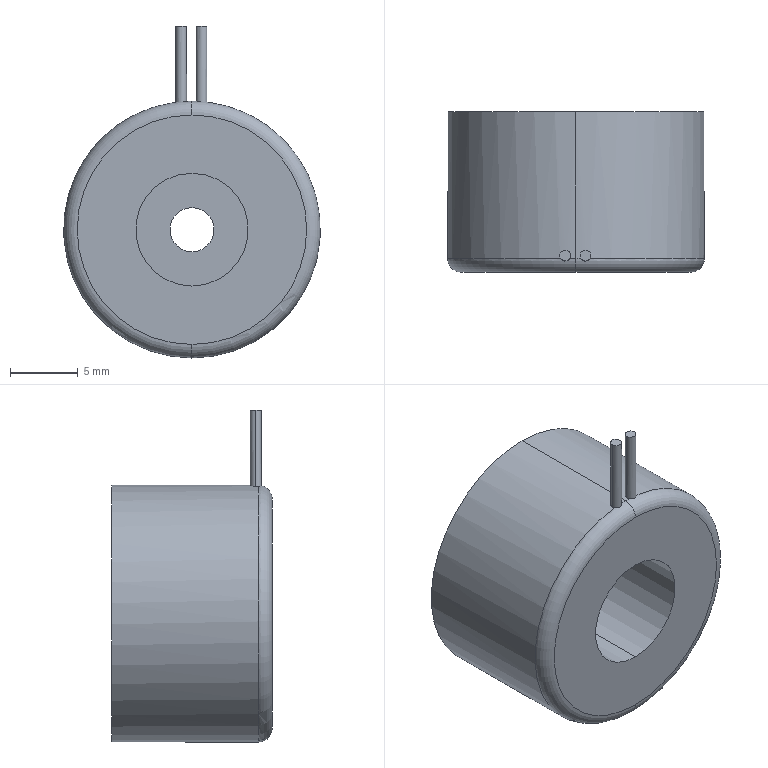Part | SolidWorks | features ICE 2, HoleWzd 1, Revolution 1 | 1 solid | 25 faces | box 18.9 x 11.8 x 24.45 mm | volume 2887 mm3 | cylinder 14 | plane 5 | cone 4 | torus 2 | commonest cylinder face diameters 0.8 x4 2.05 x4 3.25 x2 8.3 x2 18.9 x2
STEP:
#1=CARTESIAN_POINT('',(1.1,1.2,15.));
#2=VERTEX_POINT('',#1);
#3=CARTESIAN_POINT('',(0.3,1.2,15.));
#4=VERTEX_POINT('',#3);
#5=CARTESIAN_POINT('',(0.7,1.2,15.));
#6=DIRECTION('',(0.,0.,1.));
#7=DIRECTION('',(1.,0.,0.));
#8=AXIS2_PLACEMENT_3D('',#5,#6,#7);
#9=CIRCLE('',#8,0.4);
#10=EDGE_CURVE('',#2,#4,#9,.T.);
#11=ORIENTED_EDGE('',*,*,#10,.F.);
#12=CARTESIAN_POINT('',(1.1,1.2,9.386));
#13=VERTEX_POINT('',#12);
#14=CARTESIAN_POINT('',(1.1,1.2,15.));
#15=DIRECTION('',(0.,0.,-1.));
#16=VECTOR('',#15,1000.);
#17=LINE('',#14,#16);
#18=EDGE_CURVE('',#2,#13,#17,.T.);
#19=ORIENTED_EDGE('',*,*,#18,.T.);
#20=CARTESIAN_POINT('',(0.3,1.2,9.445));
#21=VERTEX_POINT('',#20);
#22=CARTESIAN_POINT('',(0.3,1.2,9.445));
#23=CARTESIAN_POINT('',(0.3,1.306,9.445));
#24=CARTESIAN_POINT('',(0.3435,1.409,9.444));
#25=CARTESIAN_POINT('',(0.4915,1.557,9.438));
#26=CARTESIAN_POINT('',(0.596,1.6,9.432));
#27=CARTESIAN_POINT('',(0.8045,1.6,9.416));
#28=CARTESIAN_POINT('',(0.9081,1.558,9.407));
#29=CARTESIAN_POINT('',(1.057,1.408,9.391));
#30=CARTESIAN_POINT('',(1.1,1.305,9.386));
#31=CARTESIAN_POINT('',(1.1,1.2,9.386));
#32=B_SPLINE_CURVE_WITH_KNOTS('',3,(#22,#23,#24,#25,#26,#27,#28,#29,#30,#31),.UNSPECIFIED.,.F.,.F.,(4,2,2,2,4),(0.,0.0003131,0.0006262,0.0009394,0.001252),.UNSPECIFIED.);
#33=EDGE_CURVE('',#21,#13,#32,.T.);
#34=ORIENTED_EDGE('',*,*,#33,.F.);
#35=CARTESIAN_POINT('',(0.3,1.2,15.));
#36=DIRECTION('',(0.,0.,-1.));
#37=VECTOR('',#36,1000.);
#38=LINE('',#35,#37);
#39=EDGE_CURVE('',#4,#21,#38,.T.);
#40=ORIENTED_EDGE('',*,*,#39,.F.);
#41=EDGE_LOOP('',(#11,#19,#34,#40));
#42=FACE_OUTER_BOUND('',#41,.T.);
#43=CARTESIAN_POINT('',(0.7,1.2,15.));
#44=DIRECTION('',(0.,0.,-1.));
#45=DIRECTION('',(-1.,0.,0.));
#46=AXIS2_PLACEMENT_3D('',#43,#44,#45);
#47=CYLINDRICAL_SURFACE('',#46,0.4);
#48=ADVANCED_FACE('',(#42),#47,.T.);
#49=CARTESIAN_POINT('',(-0.4,1.2,15.));
#50=VERTEX_POINT('',#49);
#51=CARTESIAN_POINT('',(-1.2,1.2,15.));
#52=VERTEX_POINT('',#51);
#53=CARTESIAN_POINT('',(-0.8,1.2,15.));
#54=DIRECTION('',(0.,0.,1.));
#55=DIRECTION('',(1.,0.,0.));
#56=AXIS2_PLACEMENT_3D('',#53,#54,#55);
#57=CIRCLE('',#56,0.4);
#58=EDGE_CURVE('',#50,#52,#57,.T.);
#59=ORIENTED_EDGE('',*,*,#58,.F.);
#60=CARTESIAN_POINT('',(-0.4,1.2,9.442));
#61=VERTEX_POINT('',#60);
#62=CARTESIAN_POINT('',(-0.4,1.2,15.));
#63=DIRECTION('',(0.,0.,-1.));
#64=VECTOR('',#63,1000.);
#65=LINE('',#62,#64);
#66=EDGE_CURVE('',#50,#61,#65,.T.);
#67=ORIENTED_EDGE('',*,*,#66,.T.);
#68=CARTESIAN_POINT('',(-1.2,1.2,9.373));
#69=VERTEX_POINT('',#68);
#70=CARTESIAN_POINT('',(-1.2,1.2,9.373));
#71=CARTESIAN_POINT('',(-1.2,1.306,9.373));
#72=CARTESIAN_POINT('',(-1.156,1.409,9.379));
#73=CARTESIAN_POINT('',(-1.009,1.557,9.396));
#74=CARTESIAN_POINT('',(-0.9048,1.6,9.407));
#75=CARTESIAN_POINT('',(-0.6964,1.6,9.425));
#76=CARTESIAN_POINT('',(-0.5925,1.558,9.432));
#77=CARTESIAN_POINT('',(-0.4427,1.409,9.44));
#78=CARTESIAN_POINT('',(-0.4,1.305,9.442));
#79=CARTESIAN_POINT('',(-0.4,1.2,9.442));
#80=B_SPLINE_CURVE_WITH_KNOTS('',3,(#70,#71,#72,#73,#74,#75,#76,#77,#78,#79),.UNSPECIFIED.,.F.,.F.,(4,2,2,2,4),(0.,0.0003133,0.0006265,0.0009398,0.001253),.UNSPECIFIED.);
#81=EDGE_CURVE('',#69,#61,#80,.T.);
#82=ORIENTED_EDGE('',*,*,#81,.F.);
#83=CARTESIAN_POINT('',(-1.2,1.2,15.));
#84=DIRECTION('',(0.,0.,-1.));
#85=VECTOR('',#84,1000.);
#86=LINE('',#83,#85);
#87=EDGE_CURVE('',#52,#69,#86,.T.);
#88=ORIENTED_EDGE('',*,*,#87,.F.);
#89=EDGE_LOOP('',(#59,#67,#82,#88));
#90=FACE_OUTER_BOUND('',#89,.T.);
#91=CARTESIAN_POINT('',(-0.8,1.2,15.));
#92=DIRECTION('',(0.,0.,-1.));
#93=DIRECTION('',(-1.,0.,0.));
#94=AXIS2_PLACEMENT_3D('',#91,#92,#93);
#95=CYLINDRICAL_SURFACE('',#94,0.4);
#96=ADVANCED_FACE('',(#90),#95,.T.);
#97=CARTESIAN_POINT('',(0.,7.45,-7.275));
#98=VERTEX_POINT('',#97);
#99=CARTESIAN_POINT('',(0.,7.45,-5.225));
#100=VERTEX_POINT('',#99);
#101=CARTESIAN_POINT('',(0.,7.45,-6.25));
#102=DIRECTION('',(0.,1.,0.));
#103=DIRECTION('',(0.,0.,1.));
#104=AXIS2_PLACEMENT_3D('',#101,#102,#103);
#105=CIRCLE('',#104,1.025);
#106=EDGE_CURVE('',#98,#100,#105,.T.);
#107=ORIENTED_EDGE('',*,*,#106,.F.);
#108=CARTESIAN_POINT('',(0.,11.8,-7.275));
#109=VERTEX_POINT('',#108);
#110=CARTESIAN_POINT('',(0.,11.8,-7.275));
#111=DIRECTION('',(0.,1.,0.));
#112=VECTOR('',#111,1000.);
#113=LINE('',#110,#112);
#114=EDGE_CURVE('',#98,#109,#113,.T.);
#115=ORIENTED_EDGE('',*,*,#114,.T.);
#116=CARTESIAN_POINT('',(0.,11.8,-5.225));
#117=VERTEX_POINT('',#116);
#118=CARTESIAN_POINT('',(0.,11.8,-6.25));
#119=DIRECTION('',(0.,1.,0.));
#120=DIRECTION('',(0.,0.,1.));
#121=AXIS2_PLACEMENT_3D('',#118,#119,#120);
#122=CIRCLE('',#121,1.025);
#123=EDGE_CURVE('',#109,#117,#122,.T.);
#124=ORIENTED_EDGE('',*,*,#123,.T.);
#125=CARTESIAN_POINT('',(0.,11.8,-5.225));
#126=DIRECTION('',(0.,1.,0.));
#127=VECTOR('',#126,1000.);
#128=LINE('',#125,#127);
#129=EDGE_CURVE('',#100,#117,#128,.T.);
#130=ORIENTED_EDGE('',*,*,#129,.F.);
#131=EDGE_LOOP('',(#107,#115,#124,#130));
#132=FACE_OUTER_BOUND('',#131,.T.);
#133=CARTESIAN_POINT('',(0.,11.8,-6.25));
#134=DIRECTION('',(0.,1.,0.));
#135=DIRECTION('',(0.,0.,1.));
#136=AXIS2_PLACEMENT_3D('',#133,#134,#135);
#137=CYLINDRICAL_SURFACE('',#136,1.025);
#138=ADVANCED_FACE('',(#132),#137,.F.);
#139=CARTESIAN_POINT('',(0.,6.834,-6.25));
#140=VERTEX_POINT('',#139);
#141=CARTESIAN_POINT('',(0.,7.45,-5.225));
#142=DIRECTION('',(0.,0.515,0.8572));
#143=VECTOR('',#142,1000.);
#144=LINE('',#141,#143);
#145=EDGE_CURVE('',#140,#100,#144,.T.);
#146=ORIENTED_EDGE('',*,*,#145,.F.);
#147=CARTESIAN_POINT('',(0.,7.45,-7.275));
#148=DIRECTION('',(0.,0.515,-0.8572));
#149=VECTOR('',#148,1000.);
#150=LINE('',#147,#149);
#151=EDGE_CURVE('',#140,#98,#150,.T.);
#152=ORIENTED_EDGE('',*,*,#151,.T.);
#153=ORIENTED_EDGE('',*,*,#106,.T.);
#154=EDGE_LOOP('',(#146,#152,#153));
#155=FACE_OUTER_BOUND('',#154,.T.);
#156=CARTESIAN_POINT('',(0.,7.45,-6.25));
#157=DIRECTION('',(0.,1.,0.));
#158=DIRECTION('',(0.,0.,1.));
#159=AXIS2_PLACEMENT_3D('',#156,#157,#158);
#160=CONICAL_SURFACE('',#159,1.025,1.03);
#161=ADVANCED_FACE('',(#155),#160,.F.);
#162=CARTESIAN_POINT('',(0.,7.45,5.225));
#163=VERTEX_POINT('',#162);
#164=CARTESIAN_POINT('',(0.,7.45,7.275));
#165=VERTEX_POINT('',#164);
#166=CARTESIAN_POINT('',(0.,7.45,6.25));
#167=DIRECTION('',(0.,1.,0.));
#168=DIRECTION('',(0.,0.,1.));
#169=AXIS2_PLACEMENT_3D('',#166,#167,#168);
#170=CIRCLE('',#169,1.025);
#171=EDGE_CURVE('',#163,#165,#170,.T.);
#172=ORIENTED_EDGE('',*,*,#171,.F.);
#173=CARTESIAN_POINT('',(0.,11.8,5.225));
#174=VERTEX_POINT('',#173);
#175=CARTESIAN_POINT('',(0.,11.8,5.225));
#176=DIRECTION('',(0.,1.,0.));
#177=VECTOR('',#176,1000.);
#178=LINE('',#175,#177);
#179=EDGE_CURVE('',#163,#174,#178,.T.);
#180=ORIENTED_EDGE('',*,*,#179,.T.);
#181=CARTESIAN_POINT('',(0.,11.8,7.275));
#182=VERTEX_POINT('',#181);
#183=CARTESIAN_POINT('',(0.,11.8,6.25));
#184=DIRECTION('',(0.,1.,0.));
#185=DIRECTION('',(0.,0.,1.));
#186=AXIS2_PLACEMENT_3D('',#183,#184,#185);
#187=CIRCLE('',#186,1.025);
#188=EDGE_CURVE('',#174,#182,#187,.T.);
#189=ORIENTED_EDGE('',*,*,#188,.T.);
#190=CARTESIAN_POINT('',(0.,11.8,7.275));
#191=DIRECTION('',(0.,1.,0.));
#192=VECTOR('',#191,1000.);
#193=LINE('',#190,#192);
#194=EDGE_CURVE('',#165,#182,#193,.T.);
#195=ORIENTED_EDGE('',*,*,#194,.F.);
#196=EDGE_LOOP('',(#172,#180,#189,#195));
#197=FACE_OUTER_BOUND('',#196,.T.);
#198=CARTESIAN_POINT('',(0.,11.8,6.25));
#199=DIRECTION('',(0.,1.,0.));
#200=DIRECTION('',(0.,0.,1.));
#201=AXIS2_PLACEMENT_3D('',#198,#199,#200);
#202=CYLINDRICAL_SURFACE('',#201,1.025);
#203=ADVANCED_FACE('',(#197),#202,.F.);
#204=CARTESIAN_POINT('',(0.,6.834,6.25));
#205=VERTEX_POINT('',#204);
#206=CARTESIAN_POINT('',(0.,7.45,7.275));
#207=DIRECTION('',(0.,0.515,0.8572));
#208=VECTOR('',#207,1000.);
#209=LINE('',#206,#208);
#210=EDGE_CURVE('',#205,#165,#209,.T.);
#211=ORIENTED_EDGE('',*,*,#210,.F.);
#212=CARTESIAN_POINT('',(0.,7.45,5.225));
#213=DIRECTION('',(0.,0.515,-0.8572));
#214=VECTOR('',#213,1000.);
#215=LINE('',#212,#214);
#216=EDGE_CURVE('',#205,#163,#215,.T.);
#217=ORIENTED_EDGE('',*,*,#216,.T.);
#218=ORIENTED_EDGE('',*,*,#171,.T.);
#219=EDGE_LOOP('',(#211,#217,#218));
#220=FACE_OUTER_BOUND('',#219,.T.);
#221=CARTESIAN_POINT('',(0.,7.45,6.25));
#222=DIRECTION('',(0.,1.,0.));
#223=DIRECTION('',(0.,0.,1.));
#224=AXIS2_PLACEMENT_3D('',#221,#222,#223);
#225=CONICAL_SURFACE('',#224,1.025,1.03);
#226=ADVANCED_FACE('',(#220),#225,.F.);
#227=CARTESIAN_POINT('',(0.,11.8,1.625));
#228=VERTEX_POINT('',#227);
#229=CARTESIAN_POINT('',(0.,11.8,-1.625));
#230=VERTEX_POINT('',#229);
#231=CARTESIAN_POINT('',(0.,11.8,0.));
#232=DIRECTION('',(0.,-1.,0.));
#233=DIRECTION('',(0.,0.,-1.));
#234=AXIS2_PLACEMENT_3D('',#231,#232,#233);
#235=CIRCLE('',#234,1.625);
#236=EDGE_CURVE('',#228,#230,#235,.T.);
#237=ORIENTED_EDGE('',*,*,#236,.F.);
#238=CARTESIAN_POINT('',(0.,6.3,1.625));
#239=VERTEX_POINT('',#238);
#240=CARTESIAN_POINT('',(0.,0.,1.625));
#241=DIRECTION('',(0.,-1.,0.));
#242=VECTOR('',#241,1000.);
#243=LINE('',#240,#242);
#244=EDGE_CURVE('',#228,#239,#243,.T.);
#245=ORIENTED_EDGE('',*,*,#244,.T.);
#246=CARTESIAN_POINT('',(0.,6.3,-1.625));
#247=VERTEX_POINT('',#246);
#248=CARTESIAN_POINT('',(0.,6.3,0.));
#249=DIRECTION('',(0.,-1.,0.));
#250=DIRECTION('',(0.,0.,-1.));
#251=AXIS2_PLACEMENT_3D('',#248,#249,#250);
#252=CIRCLE('',#251,1.625);
#253=EDGE_CURVE('',#239,#247,#252,.T.);
#254=ORIENTED_EDGE('',*,*,#253,.T.);
#255=CARTESIAN_POINT('',(0.,0.,-1.625));
#256=DIRECTION('',(0.,-1.,0.));
#257=VECTOR('',#256,1000.);
#258=LINE('',#255,#257);
#259=EDGE_CURVE('',#230,#247,#258,.T.);
#260=ORIENTED_EDGE('',*,*,#259,.F.);
#261=EDGE_LOOP('',(#237,#245,#254,#260));
#262=FACE_OUTER_BOUND('',#261,.T.);
#263=CARTESIAN_POINT('',(0.,0.,0.));
#264=DIRECTION('',(0.,-1.,0.));
#265=DIRECTION('',(0.,0.,-1.));
#266=AXIS2_PLACEMENT_3D('',#263,#264,#265);
#267=CYLINDRICAL_SURFACE('',#266,1.625);
#268=ADVANCED_FACE('',(#262),#267,.F.);
#269=CARTESIAN_POINT('',(0.,6.3,4.15));
#270=VERTEX_POINT('',#269);
#271=CARTESIAN_POINT('',(0.,6.3,-4.15));
#272=VERTEX_POINT('',#271);
#273=CARTESIAN_POINT('',(0.,6.3,0.));
#274=DIRECTION('',(0.,-1.,0.));
#275=DIRECTION('',(0.,0.,-1.));
#276=AXIS2_PLACEMENT_3D('',#273,#274,#275);
#277=CIRCLE('',#276,4.15);
#278=EDGE_CURVE('',#270,#272,#277,.T.);
#279=ORIENTED_EDGE('',*,*,#278,.F.);
#280=CARTESIAN_POINT('',(0.,0.,4.15));
#281=VERTEX_POINT('',#280);
#282=CARTESIAN_POINT('',(0.,0.,4.15));
#283=DIRECTION('',(0.,-1.,0.));
#284=VECTOR('',#283,1000.);
#285=LINE('',#282,#284);
#286=EDGE_CURVE('',#270,#281,#285,.T.);
#287=ORIENTED_EDGE('',*,*,#286,.T.);
#288=CARTESIAN_POINT('',(0.,0.,-4.15));
#289=VERTEX_POINT('',#288);
#290=CARTESIAN_POINT('',(0.,0.,0.));
#291=DIRECTION('',(0.,-1.,0.));
#292=DIRECTION('',(0.,0.,-1.));
#293=AXIS2_PLACEMENT_3D('',#290,#291,#292);
#294=CIRCLE('',#293,4.15);
#295=EDGE_CURVE('',#281,#289,#294,.T.);
#296=ORIENTED_EDGE('',*,*,#295,.T.);
#297=CARTESIAN_POINT('',(0.,0.,-4.15));
#298=DIRECTION('',(0.,-1.,0.));
#299=VECTOR('',#298,1000.);
#300=LINE('',#297,#299);
#301=EDGE_CURVE('',#272,#289,#300,.T.);
#302=ORIENTED_EDGE('',*,*,#301,.F.);
#303=EDGE_LOOP('',(#279,#287,#296,#302));
#304=FACE_OUTER_BOUND('',#303,.T.);
#305=CARTESIAN_POINT('',(0.,0.,0.));
#306=DIRECTION('',(0.,-1.,0.));
#307=DIRECTION('',(0.,0.,-1.));
#308=AXIS2_PLACEMENT_3D('',#305,#306,#307);
#309=CYLINDRICAL_SURFACE('',#308,4.15);
#310=ADVANCED_FACE('',(#304),#309,.F.);
#311=CARTESIAN_POINT('',(0.3536,1.,9.443));
#312=VERTEX_POINT('',#311);
#313=CARTESIAN_POINT('',(0.,1.,9.45));
#314=VERTEX_POINT('',#313);
#315=CARTESIAN_POINT('',(0.,1.,0.));
#316=DIRECTION('',(0.,-1.,0.));
#317=DIRECTION('',(0.,0.,-1.));
#318=AXIS2_PLACEMENT_3D('',#315,#316,#317);
#319=CIRCLE('',#318,9.45);
#320=EDGE_CURVE('',#312,#314,#319,.T.);
#321=ORIENTED_EDGE('',*,*,#320,.T.);
#322=CARTESIAN_POINT('',(0.,0.,8.45));
#323=VERTEX_POINT('',#322);
#324=CARTESIAN_POINT('',(0.,1.,8.45));
#325=DIRECTION('',(1.,0.,0.));
#326=DIRECTION('',(0.,0.,-1.));
#327=AXIS2_PLACEMENT_3D('',#324,#325,#326);
#328=CIRCLE('',#327,1.);
#329=EDGE_CURVE('',#314,#323,#328,.T.);
#330=ORIENTED_EDGE('',*,*,#329,.T.);
#331=CARTESIAN_POINT('',(0.,0.,-8.45));
#332=VERTEX_POINT('',#331);
#333=CARTESIAN_POINT('',(0.,0.,0.));
#334=DIRECTION('',(0.,-1.,0.));
#335=DIRECTION('',(0.,0.,-1.));
#336=AXIS2_PLACEMENT_3D('',#333,#334,#335);
#337=CIRCLE('',#336,8.45);
#338=EDGE_CURVE('',#332,#323,#337,.T.);
#339=ORIENTED_EDGE('',*,*,#338,.F.);
#340=CARTESIAN_POINT('',(0.,1.,-9.45));
#341=VERTEX_POINT('',#340);
#342=CARTESIAN_POINT('',(0.,1.,-8.45));
#343=DIRECTION('',(-1.,0.,0.));
#344=DIRECTION('',(0.,0.,1.));
#345=AXIS2_PLACEMENT_3D('',#342,#343,#344);
#346=CIRCLE('',#345,1.);
#347=EDGE_CURVE('',#341,#332,#346,.T.);
#348=ORIENTED_EDGE('',*,*,#347,.F.);
#349=CARTESIAN_POINT('',(1.046,1.,9.392));
#350=VERTEX_POINT('',#349);
#351=CARTESIAN_POINT('',(0.,1.,0.));
#352=DIRECTION('',(0.,-1.,0.));
#353=DIRECTION('',(0.,0.,-1.));
#354=AXIS2_PLACEMENT_3D('',#351,#352,#353);
#355=CIRCLE('',#354,9.45);
#356=EDGE_CURVE('',#341,#350,#355,.T.);
#357=ORIENTED_EDGE('',*,*,#356,.T.);
#358=CARTESIAN_POINT('',(1.046,1.,9.392));
#359=CARTESIAN_POINT('',(1.011,0.9389,9.396));
#360=CARTESIAN_POINT('',(0.96,0.8882,9.396));
#361=CARTESIAN_POINT('',(0.8393,0.8186,9.397));
#362=CARTESIAN_POINT('',(0.7692,0.7999,9.399));
#363=CARTESIAN_POINT('',(0.5591,0.8003,9.414));
#364=CARTESIAN_POINT('',(0.4243,0.8776,9.441));
#365=CARTESIAN_POINT('',(0.3536,1.,9.443));
#366=B_SPLINE_CURVE_WITH_KNOTS('',3,(#358,#359,#360,#361,#362,#363,#364,#365),.UNSPECIFIED.,.F.,.F.,(4,2,2,4),(0.000000228,0.0002092,0.0004181,0.0008359),.UNSPECIFIED.);
#367=EDGE_CURVE('',#350,#312,#366,.T.);
#368=ORIENTED_EDGE('',*,*,#367,.T.);
#369=EDGE_LOOP('',(#321,#330,#339,#348,#357,#368));
#370=FACE_OUTER_BOUND('',#369,.T.);
#371=CARTESIAN_POINT('',(0.,1.,0.));
#372=DIRECTION('',(0.,-1.,0.));
#373=DIRECTION('',(0.,0.,-1.));
#374=AXIS2_PLACEMENT_3D('',#371,#372,#373);
#375=TOROIDAL_SURFACE('',#374,8.45,1.);
#376=ADVANCED_FACE('',(#370),#375,.T.);
#377=CARTESIAN_POINT('',(0.,11.8,-9.45));
#378=VERTEX_POINT('',#377);
#379=CARTESIAN_POINT('',(0.,11.8,9.45));
#380=VERTEX_POINT('',#379);
#381=CARTESIAN_POINT('',(0.,11.8,0.));
#382=DIRECTION('',(0.,-1.,0.));
#383=DIRECTION('',(0.,0.,-1.));
#384=AXIS2_PLACEMENT_3D('',#381,#382,#383);
#385=CIRCLE('',#384,9.45);
#386=EDGE_CURVE('',#378,#380,#385,.T.);
#387=ORIENTED_EDGE('',*,*,#386,.T.);
#388=CARTESIAN_POINT('',(0.,0.,9.45));
#389=DIRECTION('',(0.,-1.,0.));
#390=VECTOR('',#389,1000.);
#391=LINE('',#388,#390);
#392=EDGE_CURVE('',#380,#314,#391,.T.);
#393=ORIENTED_EDGE('',*,*,#392,.T.);
#394=ORIENTED_EDGE('',*,*,#320,.F.);
#395=CARTESIAN_POINT('',(0.3536,1.,9.443));
#396=CARTESIAN_POINT('',(0.3361,1.03,9.444));
#397=CARTESIAN_POINT('',(0.3228,1.062,9.444));
#398=CARTESIAN_POINT('',(0.3047,1.13,9.445));
#399=CARTESIAN_POINT('',(0.3,1.165,9.445));
#400=CARTESIAN_POINT('',(0.3,1.2,9.445));
#401=B_SPLINE_CURVE_WITH_KNOTS('',3,(#395,#396,#397,#398,#399,#400),.UNSPECIFIED.,.F.,.F.,(4,2,4),(0.002297,0.002401,0.002505),.UNSPECIFIED.);
#402=EDGE_CURVE('',#312,#21,#401,.T.);
#403=ORIENTED_EDGE('',*,*,#402,.T.);
#404=ORIENTED_EDGE('',*,*,#33,.T.);
#405=CARTESIAN_POINT('',(1.1,1.2,9.386));
#406=CARTESIAN_POINT('',(1.1,1.165,9.386));
#407=CARTESIAN_POINT('',(1.095,1.13,9.386));
#408=CARTESIAN_POINT('',(1.077,1.062,9.388));
#409=CARTESIAN_POINT('',(1.064,1.03,9.39));
#410=CARTESIAN_POINT('',(1.046,1.,9.392));
#411=B_SPLINE_CURVE_WITH_KNOTS('',3,(#405,#406,#407,#408,#409,#410),.UNSPECIFIED.,.F.,.F.,(4,2,4),(0.001252,0.001357,0.001461),.UNSPECIFIED.);
#412=EDGE_CURVE('',#13,#350,#411,.T.);
#413=ORIENTED_EDGE('',*,*,#412,.T.);
#414=ORIENTED_EDGE('',*,*,#356,.F.);
#415=CARTESIAN_POINT('',(0.,0.,-9.45));
#416=DIRECTION('',(0.,-1.,0.));
#417=VECTOR('',#416,1000.);
#418=LINE('',#415,#417);
#419=EDGE_CURVE('',#378,#341,#418,.T.);
#420=ORIENTED_EDGE('',*,*,#419,.F.);
#421=EDGE_LOOP('',(#387,#393,#394,#403,#404,#413,#414,#420));
#422=FACE_OUTER_BOUND('',#421,.T.);
#423=CARTESIAN_POINT('',(0.,0.,0.));
#424=DIRECTION('',(0.,-1.,0.));
#425=DIRECTION('',(0.,0.,-1.));
#426=AXIS2_PLACEMENT_3D('',#423,#424,#425);
#427=CYLINDRICAL_SURFACE('',#426,9.45);
#428=ADVANCED_FACE('',(#422),#427,.T.);
#429=ORIENTED_EDGE('',*,*,#392,.F.);
#430=CARTESIAN_POINT('',(0.,11.8,0.));
#431=DIRECTION('',(0.,-1.,0.));
#432=DIRECTION('',(0.,0.,-1.));
#433=AXIS2_PLACEMENT_3D('',#430,#431,#432);
#434=CIRCLE('',#433,9.45);
#435=EDGE_CURVE('',#380,#378,#434,.T.);
#436=ORIENTED_EDGE('',*,*,#435,.T.);
#437=ORIENTED_EDGE('',*,*,#419,.T.);
#438=CARTESIAN_POINT('',(-1.146,1.,9.38));
#439=VERTEX_POINT('',#438);
#440=CARTESIAN_POINT('',(0.,1.,0.));
#441=DIRECTION('',(0.,-1.,0.));
#442=DIRECTION('',(0.,0.,-1.));
#443=AXIS2_PLACEMENT_3D('',#440,#441,#442);
#444=CIRCLE('',#443,9.45);
#445=EDGE_CURVE('',#439,#341,#444,.T.);
#446=ORIENTED_EDGE('',*,*,#445,.F.);
#447=CARTESIAN_POINT('',(-1.146,1.,9.38));
#448=CARTESIAN_POINT('',(-1.164,1.03,9.378));
#449=CARTESIAN_POINT('',(-1.177,1.062,9.376));
#450=CARTESIAN_POINT('',(-1.195,1.13,9.374));
#451=CARTESIAN_POINT('',(-1.2,1.165,9.373));
#452=CARTESIAN_POINT('',(-1.2,1.2,9.373));
#453=B_SPLINE_CURVE_WITH_KNOTS('',3,(#447,#448,#449,#450,#451,#452),.UNSPECIFIED.,.F.,.F.,(4,2,4),(0.002298,0.002402,0.002506),.UNSPECIFIED.);
#454=EDGE_CURVE('',#439,#69,#453,.T.);
#455=ORIENTED_EDGE('',*,*,#454,.T.);
#456=ORIENTED_EDGE('',*,*,#81,.T.);
#457=CARTESIAN_POINT('',(-0.4536,1.,9.439));
#458=VERTEX_POINT('',#457);
#459=CARTESIAN_POINT('',(-0.4,1.2,9.442));
#460=CARTESIAN_POINT('',(-0.4,1.165,9.442));
#461=CARTESIAN_POINT('',(-0.4046,1.13,9.441));
#462=CARTESIAN_POINT('',(-0.4227,1.062,9.441));
#463=CARTESIAN_POINT('',(-0.4361,1.03,9.44));
#464=CARTESIAN_POINT('',(-0.4536,1.,9.439));
#465=B_SPLINE_CURVE_WITH_KNOTS('',3,(#459,#460,#461,#462,#463,#464),.UNSPECIFIED.,.F.,.F.,(4,2,4),(0.001253,0.001357,0.001462),.UNSPECIFIED.);
#466=EDGE_CURVE('',#61,#458,#465,.T.);
#467=ORIENTED_EDGE('',*,*,#466,.T.);
#468=CARTESIAN_POINT('',(0.,1.,0.));
#469=DIRECTION('',(0.,-1.,0.));
#470=DIRECTION('',(0.,0.,-1.));
#471=AXIS2_PLACEMENT_3D('',#468,#469,#470);
#472=CIRCLE('',#471,9.45);
#473=EDGE_CURVE('',#314,#458,#472,.T.);
#474=ORIENTED_EDGE('',*,*,#473,.F.);
#475=EDGE_LOOP('',(#429,#436,#437,#446,#455,#456,#467,#474));
#476=FACE_OUTER_BOUND('',#475,.T.);
#477=CARTESIAN_POINT('',(0.,0.,0.));
#478=DIRECTION('',(0.,-1.,0.));
#479=DIRECTION('',(0.,0.,-1.));
#480=AXIS2_PLACEMENT_3D('',#477,#478,#479);
#481=CYLINDRICAL_SURFACE('',#480,9.45);
#482=ADVANCED_FACE('',(#476),#481,.T.);
#483=ORIENTED_EDGE('',*,*,#329,.F.);
#484=ORIENTED_EDGE('',*,*,#473,.T.);
#485=CARTESIAN_POINT('',(-0.4536,1.,9.439));
#486=CARTESIAN_POINT('',(-0.5243,0.8775,9.436));
#487=CARTESIAN_POINT('',(-0.659,0.8004,9.408));
#488=CARTESIAN_POINT('',(-0.8689,0.7998,9.39));
#489=CARTESIAN_POINT('',(-0.9387,0.8184,9.387));
#490=CARTESIAN_POINT('',(-1.06,0.8879,9.385));
#491=CARTESIAN_POINT('',(-1.111,0.9389,9.385));
#492=CARTESIAN_POINT('',(-1.146,1.,9.38));
#493=B_SPLINE_CURVE_WITH_KNOTS('',3,(#485,#486,#487,#488,#489,#490,#491,#492),.UNSPECIFIED.,.F.,.F.,(4,2,2,4),(0.000000227,0.0004183,0.0006273,0.0008363),.UNSPECIFIED.);
#494=EDGE_CURVE('',#458,#439,#493,.T.);
#495=ORIENTED_EDGE('',*,*,#494,.T.);
#496=ORIENTED_EDGE('',*,*,#445,.T.);
#497=ORIENTED_EDGE('',*,*,#347,.T.);
#498=CARTESIAN_POINT('',(0.,0.,0.));
#499=DIRECTION('',(0.,-1.,0.));
#500=DIRECTION('',(0.,0.,-1.));
#501=AXIS2_PLACEMENT_3D('',#498,#499,#500);
#502=CIRCLE('',#501,8.45);
#503=EDGE_CURVE('',#323,#332,#502,.T.);
#504=ORIENTED_EDGE('',*,*,#503,.F.);
#505=EDGE_LOOP('',(#483,#484,#495,#496,#497,#504));
#506=FACE_OUTER_BOUND('',#505,.T.);
#507=CARTESIAN_POINT('',(0.,1.,0.));
#508=DIRECTION('',(0.,-1.,0.));
#509=DIRECTION('',(0.,0.,-1.));
#510=AXIS2_PLACEMENT_3D('',#507,#508,#509);
#511=TOROIDAL_SURFACE('',#510,8.45,1.);
#512=ADVANCED_FACE('',(#506),#511,.T.);
#513=ORIENTED_EDGE('',*,*,#286,.F.);
#514=CARTESIAN_POINT('',(0.,6.3,0.));
#515=DIRECTION('',(0.,-1.,0.));
#516=DIRECTION('',(0.,0.,-1.));
#517=AXIS2_PLACEMENT_3D('',#514,#515,#516);
#518=CIRCLE('',#517,4.15);
#519=EDGE_CURVE('',#272,#270,#518,.T.);
#520=ORIENTED_EDGE('',*,*,#519,.F.);
#521=ORIENTED_EDGE('',*,*,#301,.T.);
#522=CARTESIAN_POINT('',(0.,0.,0.));
#523=DIRECTION('',(0.,-1.,0.));
#524=DIRECTION('',(0.,0.,-1.));
#525=AXIS2_PLACEMENT_3D('',#522,#523,#524);
#526=CIRCLE('',#525,4.15);
#527=EDGE_CURVE('',#289,#281,#526,.T.);
#528=ORIENTED_EDGE('',*,*,#527,.T.);
#529=EDGE_LOOP('',(#513,#520,#521,#528));
#530=FACE_OUTER_BOUND('',#529,.T.);
#531=CARTESIAN_POINT('',(0.,0.,0.));
#532=DIRECTION('',(0.,-1.,0.));
#533=DIRECTION('',(0.,0.,-1.));
#534=AXIS2_PLACEMENT_3D('',#531,#532,#533);
#535=CYLINDRICAL_SURFACE('',#534,4.15);
#536=ADVANCED_FACE('',(#530),#535,.F.);
#537=ORIENTED_EDGE('',*,*,#244,.F.);
#538=CARTESIAN_POINT('',(0.,11.8,0.));
#539=DIRECTION('',(0.,-1.,0.));
#540=DIRECTION('',(0.,0.,-1.));
#541=AXIS2_PLACEMENT_3D('',#538,#539,#540);
#542=CIRCLE('',#541,1.625);
#543=EDGE_CURVE('',#230,#228,#542,.T.);
#544=ORIENTED_EDGE('',*,*,#543,.F.);
#545=ORIENTED_EDGE('',*,*,#259,.T.);
#546=CARTESIAN_POINT('',(0.,6.3,0.));
#547=DIRECTION('',(0.,-1.,0.));
#548=DIRECTION('',(0.,0.,-1.));
#549=AXIS2_PLACEMENT_3D('',#546,#547,#548);
#550=CIRCLE('',#549,1.625);
#551=EDGE_CURVE('',#247,#239,#550,.T.);
#552=ORIENTED_EDGE('',*,*,#551,.T.);
#553=EDGE_LOOP('',(#537,#544,#545,#552));
#554=FACE_OUTER_BOUND('',#553,.T.);
#555=CARTESIAN_POINT('',(0.,0.,0.));
#556=DIRECTION('',(0.,-1.,0.));
#557=DIRECTION('',(0.,0.,-1.));
#558=AXIS2_PLACEMENT_3D('',#555,#556,#557);
#559=CYLINDRICAL_SURFACE('',#558,1.625);
#560=ADVANCED_FACE('',(#554),#559,.F.);
#561=CARTESIAN_POINT('',(0.,11.8,-6.25));
#562=DIRECTION('',(0.,1.,0.));
#563=DIRECTION('',(0.,0.,1.));
#564=AXIS2_PLACEMENT_3D('',#561,#562,#563);
#565=CIRCLE('',#564,1.025);
#566=EDGE_CURVE('',#117,#109,#565,.T.);
#567=ORIENTED_EDGE('',*,*,#566,.F.);
#568=ORIENTED_EDGE('',*,*,#123,.F.);
#569=EDGE_LOOP('',(#567,#568));
#570=FACE_BOUND('',#569,.T.);
#571=CARTESIAN_POINT('',(0.,11.8,6.25));
#572=DIRECTION('',(0.,1.,0.));
#573=DIRECTION('',(0.,0.,1.));
#574=AXIS2_PLACEMENT_3D('',#571,#572,#573);
#575=CIRCLE('',#574,1.025);
#576=EDGE_CURVE('',#182,#174,#575,.T.);
#577=ORIENTED_EDGE('',*,*,#576,.F.);
#578=ORIENTED_EDGE('',*,*,#188,.F.);
#579=EDGE_LOOP('',(#577,#578));
#580=FACE_BOUND('',#579,.T.);
#581=ORIENTED_EDGE('',*,*,#543,.T.);
#582=ORIENTED_EDGE('',*,*,#236,.T.);
#583=EDGE_LOOP('',(#581,#582));
#584=FACE_BOUND('',#583,.T.);
#585=ORIENTED_EDGE('',*,*,#386,.F.);
#586=ORIENTED_EDGE('',*,*,#435,.F.);
#587=EDGE_LOOP('',(#585,#586));
#588=FACE_OUTER_BOUND('',#587,.T.);
#589=CARTESIAN_POINT('',(1.625,11.8,0.));
#590=DIRECTION('',(0.,1.,0.));
#591=DIRECTION('',(0.,0.,1.));
#592=AXIS2_PLACEMENT_3D('',#589,#590,#591);
#593=PLANE('',#592);
#594=ADVANCED_FACE('',(#570,#580,#584,#588),#593,.T.);
#595=ORIENTED_EDGE('',*,*,#338,.T.);
#596=ORIENTED_EDGE('',*,*,#503,.T.);
#597=EDGE_LOOP('',(#595,#596));
#598=FACE_OUTER_BOUND('',#597,.T.);
#599=ORIENTED_EDGE('',*,*,#527,.F.);
#600=ORIENTED_EDGE('',*,*,#295,.F.);
#601=EDGE_LOOP('',(#599,#600));
#602=FACE_BOUND('',#601,.T.);
#603=CARTESIAN_POINT('',(8.45,0.,0.));
#604=DIRECTION('',(0.,-1.,0.));
#605=DIRECTION('',(0.,0.,-1.));
#606=AXIS2_PLACEMENT_3D('',#603,#604,#605);
#607=PLANE('',#606);
#608=ADVANCED_FACE('',(#598,#602),#607,.T.);
#609=ORIENTED_EDGE('',*,*,#519,.T.);
#610=ORIENTED_EDGE('',*,*,#278,.T.);
#611=EDGE_LOOP('',(#609,#610));
#612=FACE_OUTER_BOUND('',#611,.T.);
#613=ORIENTED_EDGE('',*,*,#551,.F.);
#614=ORIENTED_EDGE('',*,*,#253,.F.);
#615=EDGE_LOOP('',(#613,#614));
#616=FACE_BOUND('',#615,.T.);
#617=CARTESIAN_POINT('',(4.15,6.3,0.));
#618=DIRECTION('',(0.,-1.,0.));
#619=DIRECTION('',(0.,0.,-1.));
#620=AXIS2_PLACEMENT_3D('',#617,#618,#619);
#621=PLANE('',#620);
#622=ADVANCED_FACE('',(#612,#616),#621,.T.);
#623=ORIENTED_EDGE('',*,*,#216,.F.);
#624=ORIENTED_EDGE('',*,*,#210,.T.);
#625=CARTESIAN_POINT('',(0.,7.45,6.25));
#626=DIRECTION('',(0.,1.,0.));
#627=DIRECTION('',(0.,0.,1.));
#628=AXIS2_PLACEMENT_3D('',#625,#626,#627);
#629=CIRCLE('',#628,1.025);
#630=EDGE_CURVE('',#165,#163,#629,.T.);
#631=ORIENTED_EDGE('',*,*,#630,.T.);
#632=EDGE_LOOP('',(#623,#624,#631));
#633=FACE_OUTER_BOUND('',#632,.T.);
#634=CARTESIAN_POINT('',(0.,7.45,6.25));
#635=DIRECTION('',(0.,1.,0.));
#636=DIRECTION('',(0.,0.,1.));
#637=AXIS2_PLACEMENT_3D('',#634,#635,#636);
#638=CONICAL_SURFACE('',#637,1.025,1.03);
#639=ADVANCED_FACE('',(#633),#638,.F.);
#640=ORIENTED_EDGE('',*,*,#179,.F.);
#641=ORIENTED_EDGE('',*,*,#630,.F.);
#642=ORIENTED_EDGE('',*,*,#194,.T.);
#643=ORIENTED_EDGE('',*,*,#576,.T.);
#644=EDGE_LOOP('',(#640,#641,#642,#643));
#645=FACE_OUTER_BOUND('',#644,.T.);
#646=CARTESIAN_POINT('',(0.,11.8,6.25));
#647=DIRECTION('',(0.,1.,0.));
#648=DIRECTION('',(0.,0.,1.));
#649=AXIS2_PLACEMENT_3D('',#646,#647,#648);
#650=CYLINDRICAL_SURFACE('',#649,1.025);
#651=ADVANCED_FACE('',(#645),#650,.F.);
#652=ORIENTED_EDGE('',*,*,#151,.F.);
#653=ORIENTED_EDGE('',*,*,#145,.T.);
#654=CARTESIAN_POINT('',(0.,7.45,-6.25));
#655=DIRECTION('',(0.,1.,0.));
#656=DIRECTION('',(0.,0.,1.));
#657=AXIS2_PLACEMENT_3D('',#654,#655,#656);
#658=CIRCLE('',#657,1.025);
#659=EDGE_CURVE('',#100,#98,#658,.T.);
#660=ORIENTED_EDGE('',*,*,#659,.T.);
#661=EDGE_LOOP('',(#652,#653,#660));
#662=FACE_OUTER_BOUND('',#661,.T.);
#663=CARTESIAN_POINT('',(0.,7.45,-6.25));
#664=DIRECTION('',(0.,1.,0.));
#665=DIRECTION('',(0.,0.,1.));
#666=AXIS2_PLACEMENT_3D('',#663,#664,#665);
#667=CONICAL_SURFACE('',#666,1.025,1.03);
#668=ADVANCED_FACE('',(#662),#667,.F.);
#669=ORIENTED_EDGE('',*,*,#114,.F.);
#670=ORIENTED_EDGE('',*,*,#659,.F.);
#671=ORIENTED_EDGE('',*,*,#129,.T.);
#672=ORIENTED_EDGE('',*,*,#566,.T.);
#673=EDGE_LOOP('',(#669,#670,#671,#672));
#674=FACE_OUTER_BOUND('',#673,.T.);
#675=CARTESIAN_POINT('',(0.,11.8,-6.25));
#676=DIRECTION('',(0.,1.,0.));
#677=DIRECTION('',(0.,0.,1.));
#678=AXIS2_PLACEMENT_3D('',#675,#676,#677);
#679=CYLINDRICAL_SURFACE('',#678,1.025);
#680=ADVANCED_FACE('',(#674),#679,.F.);
#681=ORIENTED_EDGE('',*,*,#66,.F.);
#682=CARTESIAN_POINT('',(-0.8,1.2,15.));
#683=DIRECTION('',(0.,0.,1.));
#684=DIRECTION('',(1.,0.,0.));
#685=AXIS2_PLACEMENT_3D('',#682,#683,#684);
#686=CIRCLE('',#685,0.4);
#687=EDGE_CURVE('',#52,#50,#686,.T.);
#688=ORIENTED_EDGE('',*,*,#687,.F.);
#689=ORIENTED_EDGE('',*,*,#87,.T.);
#690=ORIENTED_EDGE('',*,*,#454,.F.);
#691=ORIENTED_EDGE('',*,*,#494,.F.);
#692=ORIENTED_EDGE('',*,*,#466,.F.);
#693=EDGE_LOOP('',(#681,#688,#689,#690,#691,#692));
#694=FACE_OUTER_BOUND('',#693,.T.);
#695=CARTESIAN_POINT('',(-0.8,1.2,15.));
#696=DIRECTION('',(0.,0.,-1.));
#697=DIRECTION('',(-1.,0.,0.));
#698=AXIS2_PLACEMENT_3D('',#695,#696,#697);
#699=CYLINDRICAL_SURFACE('',#698,0.4);
#700=ADVANCED_FACE('',(#694),#699,.T.);
#701=ORIENTED_EDGE('',*,*,#687,.T.);
#702=ORIENTED_EDGE('',*,*,#58,.T.);
#703=EDGE_LOOP('',(#701,#702));
#704=FACE_OUTER_BOUND('',#703,.T.);
#705=CARTESIAN_POINT('',(-0.8,1.2,15.));
#706=DIRECTION('',(0.,0.,1.));
#707=DIRECTION('',(1.,0.,0.));
#708=AXIS2_PLACEMENT_3D('',#705,#706,#707);
#709=PLANE('',#708);
#710=ADVANCED_FACE('',(#704),#709,.T.);
#711=ORIENTED_EDGE('',*,*,#18,.F.);
#712=CARTESIAN_POINT('',(0.7,1.2,15.));
#713=DIRECTION('',(0.,0.,1.));
#714=DIRECTION('',(1.,0.,0.));
#715=AXIS2_PLACEMENT_3D('',#712,#713,#714);
#716=CIRCLE('',#715,0.4);
#717=EDGE_CURVE('',#4,#2,#716,.T.);
#718=ORIENTED_EDGE('',*,*,#717,.F.);
#719=ORIENTED_EDGE('',*,*,#39,.T.);
#720=ORIENTED_EDGE('',*,*,#402,.F.);
#721=ORIENTED_EDGE('',*,*,#367,.F.);
#722=ORIENTED_EDGE('',*,*,#412,.F.);
#723=EDGE_LOOP('',(#711,#718,#719,#720,#721,#722));
#724=FACE_OUTER_BOUND('',#723,.T.);
#725=CARTESIAN_POINT('',(0.7,1.2,15.));
#726=DIRECTION('',(0.,0.,-1.));
#727=DIRECTION('',(-1.,0.,0.));
#728=AXIS2_PLACEMENT_3D('',#725,#726,#727);
#729=CYLINDRICAL_SURFACE('',#728,0.4);
#730=ADVANCED_FACE('',(#724),#729,.T.);
#731=ORIENTED_EDGE('',*,*,#717,.T.);
#732=ORIENTED_EDGE('',*,*,#10,.T.);
#733=EDGE_LOOP('',(#731,#732));
#734=FACE_OUTER_BOUND('',#733,.T.);
#735=CARTESIAN_POINT('',(0.7,1.2,15.));
#736=DIRECTION('',(0.,0.,1.));
#737=DIRECTION('',(1.,0.,0.));
#738=AXIS2_PLACEMENT_3D('',#735,#736,#737);
#739=PLANE('',#738);
#740=ADVANCED_FACE('',(#734),#739,.T.);
#741=CLOSED_SHELL('',(#48,#96,#138,#161,#203,#226,#268,#310,#376,#428,#482,#512,#536,#560,#594,#608,#622,#639,#651,#668,#680,#700,#710,#730,#740));
#742=MANIFOLD_SOLID_BREP('',#741);
#743=CARTESIAN_POINT('',(0.,0.,0.));
#744=DIRECTION('',(0.,0.,1.));
#745=DIRECTION('',(1.,0.,0.));
#746=AXIS2_PLACEMENT_3D('',#743,#744,#745);
#747=(LENGTH_UNIT()NAMED_UNIT(*)SI_UNIT(.MILLI.,.METRE.));
#748=UNCERTAINTY_MEASURE_WITH_UNIT(LENGTH_MEASURE(0.00001),#747,'','');
#749=(NAMED_UNIT(*)PLANE_ANGLE_UNIT()SI_UNIT($,.RADIAN.));
#750=(NAMED_UNIT(*)SI_UNIT($,.STERADIAN.)SOLID_ANGLE_UNIT());
#751=(GEOMETRIC_REPRESENTATION_CONTEXT(3)GLOBAL_UNCERTAINTY_ASSIGNED_CONTEXT((#748))GLOBAL_UNIT_ASSIGNED_CONTEXT((#747,#749,#750))REPRESENTATION_CONTEXT('',''));
#752=ADVANCED_BREP_SHAPE_REPRESENTATION('',(#742,#746),#751);